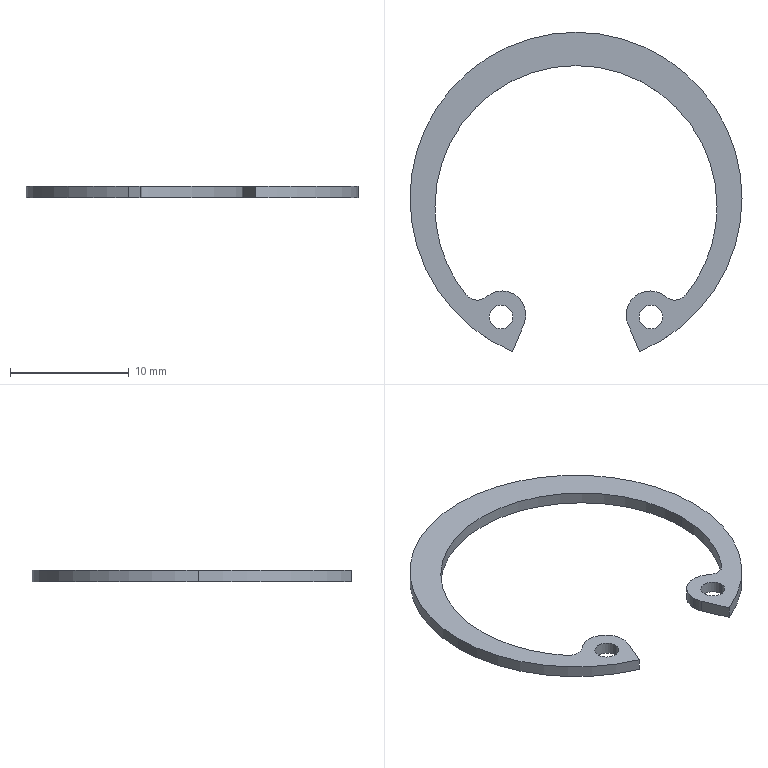Part | SolidWorks | features Extrusion 1 | 1 solid | 19 faces | box 27.9 x 26.838 x 1 mm | volume 169.048 mm3 | cylinder 15 | plane 4 | commonest cylinder face diameters 2 x4 4 x3 23.7 x3 27.9 x3 2.4 x2
STEP:
#1=CARTESIAN_POINT('',(5.298,-9.979,1.));
#2=VERTEX_POINT('',#1);
#3=CARTESIAN_POINT('',(7.298,-9.979,1.));
#4=VERTEX_POINT('',#3);
#5=CARTESIAN_POINT('',(6.298,-9.979,1.));
#6=DIRECTION('',(0.,0.,1.));
#7=DIRECTION('',(-1.,0.,0.));
#8=AXIS2_PLACEMENT_3D('',#5,#6,#7);
#9=CIRCLE('',#8,1.);
#10=EDGE_CURVE('',#2,#4,#9,.T.);
#11=ORIENTED_EDGE('',*,*,#10,.T.);
#12=CARTESIAN_POINT('',(7.298,-9.979,0.));
#13=VERTEX_POINT('',#12);
#14=CARTESIAN_POINT('',(7.298,-9.979,1.));
#15=DIRECTION('',(0.,0.,-1.));
#16=VECTOR('',#15,1000.);
#17=LINE('',#14,#16);
#18=EDGE_CURVE('',#4,#13,#17,.T.);
#19=ORIENTED_EDGE('',*,*,#18,.T.);
#20=CARTESIAN_POINT('',(5.298,-9.979,0.));
#21=VERTEX_POINT('',#20);
#22=CARTESIAN_POINT('',(6.298,-9.979,0.));
#23=DIRECTION('',(0.,0.,1.));
#24=DIRECTION('',(-1.,0.,0.));
#25=AXIS2_PLACEMENT_3D('',#22,#23,#24);
#26=CIRCLE('',#25,1.);
#27=EDGE_CURVE('',#21,#13,#26,.T.);
#28=ORIENTED_EDGE('',*,*,#27,.F.);
#29=CARTESIAN_POINT('',(5.298,-9.979,1.));
#30=DIRECTION('',(0.,0.,-1.));
#31=VECTOR('',#30,1000.);
#32=LINE('',#29,#31);
#33=EDGE_CURVE('',#2,#21,#32,.T.);
#34=ORIENTED_EDGE('',*,*,#33,.F.);
#35=EDGE_LOOP('',(#11,#19,#28,#34));
#36=FACE_OUTER_BOUND('',#35,.T.);
#37=CARTESIAN_POINT('',(6.298,-9.979,1.));
#38=DIRECTION('',(0.,0.,-1.));
#39=DIRECTION('',(-1.,0.,0.));
#40=AXIS2_PLACEMENT_3D('',#37,#38,#39);
#41=CYLINDRICAL_SURFACE('',#40,1.);
#42=ADVANCED_FACE('',(#36),#41,.F.);
#43=CARTESIAN_POINT('',(-7.298,-9.979,1.));
#44=VERTEX_POINT('',#43);
#45=CARTESIAN_POINT('',(-5.298,-9.979,1.));
#46=VERTEX_POINT('',#45);
#47=CARTESIAN_POINT('',(-6.298,-9.979,1.));
#48=DIRECTION('',(0.,0.,1.));
#49=DIRECTION('',(1.,0.,0.));
#50=AXIS2_PLACEMENT_3D('',#47,#48,#49);
#51=CIRCLE('',#50,1.);
#52=EDGE_CURVE('',#44,#46,#51,.T.);
#53=ORIENTED_EDGE('',*,*,#52,.T.);
#54=CARTESIAN_POINT('',(-5.298,-9.979,0.));
#55=VERTEX_POINT('',#54);
#56=CARTESIAN_POINT('',(-5.298,-9.979,1.));
#57=DIRECTION('',(0.,0.,-1.));
#58=VECTOR('',#57,1000.);
#59=LINE('',#56,#58);
#60=EDGE_CURVE('',#46,#55,#59,.T.);
#61=ORIENTED_EDGE('',*,*,#60,.T.);
#62=CARTESIAN_POINT('',(-7.298,-9.979,0.));
#63=VERTEX_POINT('',#62);
#64=CARTESIAN_POINT('',(-6.298,-9.979,0.));
#65=DIRECTION('',(0.,0.,1.));
#66=DIRECTION('',(1.,0.,0.));
#67=AXIS2_PLACEMENT_3D('',#64,#65,#66);
#68=CIRCLE('',#67,1.);
#69=EDGE_CURVE('',#63,#55,#68,.T.);
#70=ORIENTED_EDGE('',*,*,#69,.F.);
#71=CARTESIAN_POINT('',(-7.298,-9.979,1.));
#72=DIRECTION('',(0.,0.,-1.));
#73=VECTOR('',#72,1000.);
#74=LINE('',#71,#73);
#75=EDGE_CURVE('',#44,#63,#74,.T.);
#76=ORIENTED_EDGE('',*,*,#75,.F.);
#77=EDGE_LOOP('',(#53,#61,#70,#76));
#78=FACE_OUTER_BOUND('',#77,.T.);
#79=CARTESIAN_POINT('',(-6.298,-9.979,1.));
#80=DIRECTION('',(0.,0.,-1.));
#81=DIRECTION('',(-1.,0.,0.));
#82=AXIS2_PLACEMENT_3D('',#79,#80,#81);
#83=CYLINDRICAL_SURFACE('',#82,1.);
#84=ADVANCED_FACE('',(#78),#83,.F.);
#85=CARTESIAN_POINT('',(13.95,0.,1.));
#86=VERTEX_POINT('',#85);
#87=CARTESIAN_POINT('',(-13.95,0.,1.));
#88=VERTEX_POINT('',#87);
#89=CARTESIAN_POINT('',(0.,0.,1.));
#90=DIRECTION('',(0.,0.,1.));
#91=DIRECTION('',(1.,0.,0.));
#92=AXIS2_PLACEMENT_3D('',#89,#90,#91);
#93=CIRCLE('',#92,13.95);
#94=EDGE_CURVE('',#86,#88,#93,.T.);
#95=ORIENTED_EDGE('',*,*,#94,.F.);
#96=CARTESIAN_POINT('',(13.95,0.,0.));
#97=VERTEX_POINT('',#96);
#98=CARTESIAN_POINT('',(13.95,0.,1.));
#99=DIRECTION('',(0.,0.,-1.));
#100=VECTOR('',#99,1000.);
#101=LINE('',#98,#100);
#102=EDGE_CURVE('',#86,#97,#101,.T.);
#103=ORIENTED_EDGE('',*,*,#102,.T.);
#104=CARTESIAN_POINT('',(-13.95,0.,0.));
#105=VERTEX_POINT('',#104);
#106=CARTESIAN_POINT('',(0.,0.,0.));
#107=DIRECTION('',(0.,0.,1.));
#108=DIRECTION('',(1.,0.,0.));
#109=AXIS2_PLACEMENT_3D('',#106,#107,#108);
#110=CIRCLE('',#109,13.95);
#111=EDGE_CURVE('',#97,#105,#110,.T.);
#112=ORIENTED_EDGE('',*,*,#111,.T.);
#113=CARTESIAN_POINT('',(-13.95,0.,1.));
#114=DIRECTION('',(0.,0.,-1.));
#115=VECTOR('',#114,1000.);
#116=LINE('',#113,#115);
#117=EDGE_CURVE('',#88,#105,#116,.T.);
#118=ORIENTED_EDGE('',*,*,#117,.F.);
#119=EDGE_LOOP('',(#95,#103,#112,#118));
#120=FACE_OUTER_BOUND('',#119,.T.);
#121=CARTESIAN_POINT('',(0.,0.,1.));
#122=DIRECTION('',(0.,0.,-1.));
#123=DIRECTION('',(-1.,0.,0.));
#124=AXIS2_PLACEMENT_3D('',#121,#122,#123);
#125=CYLINDRICAL_SURFACE('',#124,13.95);
#126=ADVANCED_FACE('',(#120),#125,.T.);
#127=CARTESIAN_POINT('',(-5.338,-12.888,1.));
#128=VERTEX_POINT('',#127);
#129=CARTESIAN_POINT('',(0.,0.,1.));
#130=DIRECTION('',(0.,0.,1.));
#131=DIRECTION('',(1.,0.,0.));
#132=AXIS2_PLACEMENT_3D('',#129,#130,#131);
#133=CIRCLE('',#132,13.95);
#134=EDGE_CURVE('',#88,#128,#133,.T.);
#135=ORIENTED_EDGE('',*,*,#134,.F.);
#136=ORIENTED_EDGE('',*,*,#117,.T.);
#137=CARTESIAN_POINT('',(-5.338,-12.888,0.));
#138=VERTEX_POINT('',#137);
#139=CARTESIAN_POINT('',(0.,0.,0.));
#140=DIRECTION('',(0.,0.,1.));
#141=DIRECTION('',(1.,0.,0.));
#142=AXIS2_PLACEMENT_3D('',#139,#140,#141);
#143=CIRCLE('',#142,13.95);
#144=EDGE_CURVE('',#105,#138,#143,.T.);
#145=ORIENTED_EDGE('',*,*,#144,.T.);
#146=CARTESIAN_POINT('',(-5.338,-12.888,1.));
#147=DIRECTION('',(0.,0.,-1.));
#148=VECTOR('',#147,1000.);
#149=LINE('',#146,#148);
#150=EDGE_CURVE('',#128,#138,#149,.T.);
#151=ORIENTED_EDGE('',*,*,#150,.F.);
#152=EDGE_LOOP('',(#135,#136,#145,#151));
#153=FACE_OUTER_BOUND('',#152,.T.);
#154=CARTESIAN_POINT('',(0.,0.,1.));
#155=DIRECTION('',(0.,0.,-1.));
#156=DIRECTION('',(-1.,0.,0.));
#157=AXIS2_PLACEMENT_3D('',#154,#155,#156);
#158=CYLINDRICAL_SURFACE('',#157,13.95);
#159=ADVANCED_FACE('',(#153),#158,.T.);
#160=CARTESIAN_POINT('',(4.217,-9.782,1.));
#161=VERTEX_POINT('',#160);
#162=CARTESIAN_POINT('',(4.369,-10.547,1.));
#163=VERTEX_POINT('',#162);
#164=CARTESIAN_POINT('',(6.217,-9.782,1.));
#165=DIRECTION('',(0.,0.,1.));
#166=DIRECTION('',(-1.,0.,0.));
#167=AXIS2_PLACEMENT_3D('',#164,#165,#166);
#168=CIRCLE('',#167,2.);
#169=EDGE_CURVE('',#161,#163,#168,.T.);
#170=ORIENTED_EDGE('',*,*,#169,.F.);
#171=CARTESIAN_POINT('',(4.217,-9.782,0.));
#172=VERTEX_POINT('',#171);
#173=CARTESIAN_POINT('',(4.217,-9.782,1.));
#174=DIRECTION('',(0.,0.,-1.));
#175=VECTOR('',#174,1000.);
#176=LINE('',#173,#175);
#177=EDGE_CURVE('',#161,#172,#176,.T.);
#178=ORIENTED_EDGE('',*,*,#177,.T.);
#179=CARTESIAN_POINT('',(4.369,-10.547,0.));
#180=VERTEX_POINT('',#179);
#181=CARTESIAN_POINT('',(6.217,-9.782,0.));
#182=DIRECTION('',(0.,0.,1.));
#183=DIRECTION('',(-1.,0.,0.));
#184=AXIS2_PLACEMENT_3D('',#181,#182,#183);
#185=CIRCLE('',#184,2.);
#186=EDGE_CURVE('',#172,#180,#185,.T.);
#187=ORIENTED_EDGE('',*,*,#186,.T.);
#188=CARTESIAN_POINT('',(4.369,-10.547,1.));
#189=DIRECTION('',(0.,0.,-1.));
#190=VECTOR('',#189,1000.);
#191=LINE('',#188,#190);
#192=EDGE_CURVE('',#163,#180,#191,.T.);
#193=ORIENTED_EDGE('',*,*,#192,.F.);
#194=EDGE_LOOP('',(#170,#178,#187,#193));
#195=FACE_OUTER_BOUND('',#194,.T.);
#196=CARTESIAN_POINT('',(6.217,-9.782,1.));
#197=DIRECTION('',(0.,0.,-1.));
#198=DIRECTION('',(-1.,0.,0.));
#199=AXIS2_PLACEMENT_3D('',#196,#197,#198);
#200=CYLINDRICAL_SURFACE('',#199,2.);
#201=ADVANCED_FACE('',(#195),#200,.T.);
#202=CARTESIAN_POINT('',(11.85,-0.7,1.));
#203=VERTEX_POINT('',#202);
#204=CARTESIAN_POINT('',(9.246,-8.112,1.));
#205=VERTEX_POINT('',#204);
#206=CARTESIAN_POINT('',(0.,-0.7,1.));
#207=DIRECTION('',(0.,0.,-1.));
#208=DIRECTION('',(1.,0.,0.));
#209=AXIS2_PLACEMENT_3D('',#206,#207,#208);
#210=CIRCLE('',#209,11.85);
#211=EDGE_CURVE('',#203,#205,#210,.T.);
#212=ORIENTED_EDGE('',*,*,#211,.F.);
#213=CARTESIAN_POINT('',(11.85,-0.7,0.));
#214=VERTEX_POINT('',#213);
#215=CARTESIAN_POINT('',(11.85,-0.7,1.));
#216=DIRECTION('',(0.,0.,-1.));
#217=VECTOR('',#216,1000.);
#218=LINE('',#215,#217);
#219=EDGE_CURVE('',#203,#214,#218,.T.);
#220=ORIENTED_EDGE('',*,*,#219,.T.);
#221=CARTESIAN_POINT('',(9.246,-8.112,0.));
#222=VERTEX_POINT('',#221);
#223=CARTESIAN_POINT('',(0.,-0.7,0.));
#224=DIRECTION('',(0.,0.,-1.));
#225=DIRECTION('',(1.,0.,0.));
#226=AXIS2_PLACEMENT_3D('',#223,#224,#225);
#227=CIRCLE('',#226,11.85);
#228=EDGE_CURVE('',#214,#222,#227,.T.);
#229=ORIENTED_EDGE('',*,*,#228,.T.);
#230=CARTESIAN_POINT('',(9.246,-8.112,1.));
#231=DIRECTION('',(0.,0.,-1.));
#232=VECTOR('',#231,1000.);
#233=LINE('',#230,#232);
#234=EDGE_CURVE('',#205,#222,#233,.T.);
#235=ORIENTED_EDGE('',*,*,#234,.F.);
#236=EDGE_LOOP('',(#212,#220,#229,#235));
#237=FACE_OUTER_BOUND('',#236,.T.);
#238=CARTESIAN_POINT('',(0.,-0.7,1.));
#239=DIRECTION('',(0.,0.,-1.));
#240=DIRECTION('',(-1.,0.,0.));
#241=AXIS2_PLACEMENT_3D('',#238,#239,#240);
#242=CYLINDRICAL_SURFACE('',#241,11.85);
#243=ADVANCED_FACE('',(#237),#242,.F.);
#244=ORIENTED_EDGE('',*,*,#219,.F.);
#245=CARTESIAN_POINT('',(-11.85,-0.7,1.));
#246=VERTEX_POINT('',#245);
#247=CARTESIAN_POINT('',(0.,-0.7,1.));
#248=DIRECTION('',(0.,0.,-1.));
#249=DIRECTION('',(1.,0.,0.));
#250=AXIS2_PLACEMENT_3D('',#247,#248,#249);
#251=CIRCLE('',#250,11.85);
#252=EDGE_CURVE('',#246,#203,#251,.T.);
#253=ORIENTED_EDGE('',*,*,#252,.F.);
#254=CARTESIAN_POINT('',(-11.85,-0.7,0.));
#255=VERTEX_POINT('',#254);
#256=CARTESIAN_POINT('',(-11.85,-0.7,1.));
#257=DIRECTION('',(0.,0.,-1.));
#258=VECTOR('',#257,1000.);
#259=LINE('',#256,#258);
#260=EDGE_CURVE('',#246,#255,#259,.T.);
#261=ORIENTED_EDGE('',*,*,#260,.T.);
#262=CARTESIAN_POINT('',(0.,-0.7,0.));
#263=DIRECTION('',(0.,0.,-1.));
#264=DIRECTION('',(1.,0.,0.));
#265=AXIS2_PLACEMENT_3D('',#262,#263,#264);
#266=CIRCLE('',#265,11.85);
#267=EDGE_CURVE('',#255,#214,#266,.T.);
#268=ORIENTED_EDGE('',*,*,#267,.T.);
#269=EDGE_LOOP('',(#244,#253,#261,#268));
#270=FACE_OUTER_BOUND('',#269,.T.);
#271=CARTESIAN_POINT('',(0.,-0.7,1.));
#272=DIRECTION('',(0.,0.,-1.));
#273=DIRECTION('',(-1.,0.,0.));
#274=AXIS2_PLACEMENT_3D('',#271,#272,#273);
#275=CYLINDRICAL_SURFACE('',#274,11.85);
#276=ADVANCED_FACE('',(#270),#275,.F.);
#277=ORIENTED_EDGE('',*,*,#52,.F.);
#278=CARTESIAN_POINT('',(-6.298,-9.979,1.));
#279=DIRECTION('',(0.,0.,1.));
#280=DIRECTION('',(1.,0.,0.));
#281=AXIS2_PLACEMENT_3D('',#278,#279,#280);
#282=CIRCLE('',#281,1.);
#283=EDGE_CURVE('',#46,#44,#282,.T.);
#284=ORIENTED_EDGE('',*,*,#283,.F.);
#285=EDGE_LOOP('',(#277,#284));
#286=FACE_BOUND('',#285,.T.);
#287=CARTESIAN_POINT('',(-4.369,-10.547,1.));
#288=VERTEX_POINT('',#287);
#289=CARTESIAN_POINT('',(-7.525,-8.269,1.));
#290=VERTEX_POINT('',#289);
#291=CARTESIAN_POINT('',(-6.217,-9.782,1.));
#292=DIRECTION('',(0.,0.,1.));
#293=DIRECTION('',(1.,0.,0.));
#294=AXIS2_PLACEMENT_3D('',#291,#292,#293);
#295=CIRCLE('',#294,2.);
#296=EDGE_CURVE('',#288,#290,#295,.T.);
#297=ORIENTED_EDGE('',*,*,#296,.T.);
#298=CARTESIAN_POINT('',(-9.246,-8.112,1.));
#299=VERTEX_POINT('',#298);
#300=CARTESIAN_POINT('',(-8.31,-7.361,1.));
#301=DIRECTION('',(0.,0.,-1.));
#302=DIRECTION('',(-1.,0.,0.));
#303=AXIS2_PLACEMENT_3D('',#300,#301,#302);
#304=CIRCLE('',#303,1.2);
#305=EDGE_CURVE('',#290,#299,#304,.T.);
#306=ORIENTED_EDGE('',*,*,#305,.T.);
#307=CARTESIAN_POINT('',(0.,-0.7,1.));
#308=DIRECTION('',(0.,0.,-1.));
#309=DIRECTION('',(1.,0.,0.));
#310=AXIS2_PLACEMENT_3D('',#307,#308,#309);
#311=CIRCLE('',#310,11.85);
#312=EDGE_CURVE('',#299,#246,#311,.T.);
#313=ORIENTED_EDGE('',*,*,#312,.T.);
#314=ORIENTED_EDGE('',*,*,#252,.T.);
#315=ORIENTED_EDGE('',*,*,#211,.T.);
#316=CARTESIAN_POINT('',(7.525,-8.269,1.));
#317=VERTEX_POINT('',#316);
#318=CARTESIAN_POINT('',(8.31,-7.361,1.));
#319=DIRECTION('',(0.,0.,-1.));
#320=DIRECTION('',(1.,0.,0.));
#321=AXIS2_PLACEMENT_3D('',#318,#319,#320);
#322=CIRCLE('',#321,1.2);
#323=EDGE_CURVE('',#205,#317,#322,.T.);
#324=ORIENTED_EDGE('',*,*,#323,.T.);
#325=CARTESIAN_POINT('',(6.217,-9.782,1.));
#326=DIRECTION('',(0.,0.,1.));
#327=DIRECTION('',(-1.,0.,0.));
#328=AXIS2_PLACEMENT_3D('',#325,#326,#327);
#329=CIRCLE('',#328,2.);
#330=EDGE_CURVE('',#317,#161,#329,.T.);
#331=ORIENTED_EDGE('',*,*,#330,.T.);
#332=ORIENTED_EDGE('',*,*,#169,.T.);
#333=CARTESIAN_POINT('',(5.338,-12.888,1.));
#334=VERTEX_POINT('',#333);
#335=CARTESIAN_POINT('',(4.369,-10.547,1.));
#336=DIRECTION('',(0.3827,-0.9239,0.));
#337=VECTOR('',#336,1000.);
#338=LINE('',#335,#337);
#339=EDGE_CURVE('',#163,#334,#338,.T.);
#340=ORIENTED_EDGE('',*,*,#339,.T.);
#341=CARTESIAN_POINT('',(0.,0.,1.));
#342=DIRECTION('',(0.,0.,1.));
#343=DIRECTION('',(1.,0.,0.));
#344=AXIS2_PLACEMENT_3D('',#341,#342,#343);
#345=CIRCLE('',#344,13.95);
#346=EDGE_CURVE('',#334,#86,#345,.T.);
#347=ORIENTED_EDGE('',*,*,#346,.T.);
#348=ORIENTED_EDGE('',*,*,#94,.T.);
#349=ORIENTED_EDGE('',*,*,#134,.T.);
#350=CARTESIAN_POINT('',(-4.369,-10.547,1.));
#351=DIRECTION('',(0.3827,0.9239,0.));
#352=VECTOR('',#351,1000.);
#353=LINE('',#350,#352);
#354=EDGE_CURVE('',#128,#288,#353,.T.);
#355=ORIENTED_EDGE('',*,*,#354,.T.);
#356=EDGE_LOOP('',(#297,#306,#313,#314,#315,#324,#331,#332,#340,#347,#348,#349,#355));
#357=FACE_OUTER_BOUND('',#356,.T.);
#358=ORIENTED_EDGE('',*,*,#10,.F.);
#359=CARTESIAN_POINT('',(6.298,-9.979,1.));
#360=DIRECTION('',(0.,0.,1.));
#361=DIRECTION('',(-1.,0.,0.));
#362=AXIS2_PLACEMENT_3D('',#359,#360,#361);
#363=CIRCLE('',#362,1.);
#364=EDGE_CURVE('',#4,#2,#363,.T.);
#365=ORIENTED_EDGE('',*,*,#364,.F.);
#366=EDGE_LOOP('',(#358,#365));
#367=FACE_BOUND('',#366,.T.);
#368=CARTESIAN_POINT('',(-6.217,-9.782,1.));
#369=DIRECTION('',(0.,0.,1.));
#370=DIRECTION('',(1.,0.,0.));
#371=AXIS2_PLACEMENT_3D('',#368,#369,#370);
#372=PLANE('',#371);
#373=ADVANCED_FACE('',(#286,#357,#367),#372,.T.);
#374=CARTESIAN_POINT('',(-4.369,-10.547,0.));
#375=VERTEX_POINT('',#374);
#376=CARTESIAN_POINT('',(-7.525,-8.269,0.));
#377=VERTEX_POINT('',#376);
#378=CARTESIAN_POINT('',(-6.217,-9.782,0.));
#379=DIRECTION('',(0.,0.,1.));
#380=DIRECTION('',(1.,0.,0.));
#381=AXIS2_PLACEMENT_3D('',#378,#379,#380);
#382=CIRCLE('',#381,2.);
#383=EDGE_CURVE('',#375,#377,#382,.T.);
#384=ORIENTED_EDGE('',*,*,#383,.F.);
#385=CARTESIAN_POINT('',(-4.369,-10.547,0.));
#386=DIRECTION('',(0.3827,0.9239,0.));
#387=VECTOR('',#386,1000.);
#388=LINE('',#385,#387);
#389=EDGE_CURVE('',#138,#375,#388,.T.);
#390=ORIENTED_EDGE('',*,*,#389,.F.);
#391=ORIENTED_EDGE('',*,*,#144,.F.);
#392=ORIENTED_EDGE('',*,*,#111,.F.);
#393=CARTESIAN_POINT('',(5.338,-12.888,0.));
#394=VERTEX_POINT('',#393);
#395=CARTESIAN_POINT('',(0.,0.,0.));
#396=DIRECTION('',(0.,0.,1.));
#397=DIRECTION('',(1.,0.,0.));
#398=AXIS2_PLACEMENT_3D('',#395,#396,#397);
#399=CIRCLE('',#398,13.95);
#400=EDGE_CURVE('',#394,#97,#399,.T.);
#401=ORIENTED_EDGE('',*,*,#400,.F.);
#402=CARTESIAN_POINT('',(4.369,-10.547,0.));
#403=DIRECTION('',(0.3827,-0.9239,0.));
#404=VECTOR('',#403,1000.);
#405=LINE('',#402,#404);
#406=EDGE_CURVE('',#180,#394,#405,.T.);
#407=ORIENTED_EDGE('',*,*,#406,.F.);
#408=ORIENTED_EDGE('',*,*,#186,.F.);
#409=CARTESIAN_POINT('',(7.525,-8.269,0.));
#410=VERTEX_POINT('',#409);
#411=CARTESIAN_POINT('',(6.217,-9.782,0.));
#412=DIRECTION('',(0.,0.,1.));
#413=DIRECTION('',(-1.,0.,0.));
#414=AXIS2_PLACEMENT_3D('',#411,#412,#413);
#415=CIRCLE('',#414,2.);
#416=EDGE_CURVE('',#410,#172,#415,.T.);
#417=ORIENTED_EDGE('',*,*,#416,.F.);
#418=CARTESIAN_POINT('',(8.31,-7.361,0.));
#419=DIRECTION('',(0.,0.,-1.));
#420=DIRECTION('',(1.,0.,0.));
#421=AXIS2_PLACEMENT_3D('',#418,#419,#420);
#422=CIRCLE('',#421,1.2);
#423=EDGE_CURVE('',#222,#410,#422,.T.);
#424=ORIENTED_EDGE('',*,*,#423,.F.);
#425=ORIENTED_EDGE('',*,*,#228,.F.);
#426=ORIENTED_EDGE('',*,*,#267,.F.);
#427=CARTESIAN_POINT('',(-9.246,-8.112,0.));
#428=VERTEX_POINT('',#427);
#429=CARTESIAN_POINT('',(0.,-0.7,0.));
#430=DIRECTION('',(0.,0.,-1.));
#431=DIRECTION('',(1.,0.,0.));
#432=AXIS2_PLACEMENT_3D('',#429,#430,#431);
#433=CIRCLE('',#432,11.85);
#434=EDGE_CURVE('',#428,#255,#433,.T.);
#435=ORIENTED_EDGE('',*,*,#434,.F.);
#436=CARTESIAN_POINT('',(-8.31,-7.361,0.));
#437=DIRECTION('',(0.,0.,-1.));
#438=DIRECTION('',(-1.,0.,0.));
#439=AXIS2_PLACEMENT_3D('',#436,#437,#438);
#440=CIRCLE('',#439,1.2);
#441=EDGE_CURVE('',#377,#428,#440,.T.);
#442=ORIENTED_EDGE('',*,*,#441,.F.);
#443=EDGE_LOOP('',(#384,#390,#391,#392,#401,#407,#408,#417,#424,#425,#426,#435,#442));
#444=FACE_OUTER_BOUND('',#443,.T.);
#445=ORIENTED_EDGE('',*,*,#69,.T.);
#446=CARTESIAN_POINT('',(-6.298,-9.979,0.));
#447=DIRECTION('',(0.,0.,1.));
#448=DIRECTION('',(1.,0.,0.));
#449=AXIS2_PLACEMENT_3D('',#446,#447,#448);
#450=CIRCLE('',#449,1.);
#451=EDGE_CURVE('',#55,#63,#450,.T.);
#452=ORIENTED_EDGE('',*,*,#451,.T.);
#453=EDGE_LOOP('',(#445,#452));
#454=FACE_BOUND('',#453,.T.);
#455=ORIENTED_EDGE('',*,*,#27,.T.);
#456=CARTESIAN_POINT('',(6.298,-9.979,0.));
#457=DIRECTION('',(0.,0.,1.));
#458=DIRECTION('',(-1.,0.,0.));
#459=AXIS2_PLACEMENT_3D('',#456,#457,#458);
#460=CIRCLE('',#459,1.);
#461=EDGE_CURVE('',#13,#21,#460,.T.);
#462=ORIENTED_EDGE('',*,*,#461,.T.);
#463=EDGE_LOOP('',(#455,#462));
#464=FACE_BOUND('',#463,.T.);
#465=CARTESIAN_POINT('',(-6.217,-9.782,0.));
#466=DIRECTION('',(0.,0.,1.));
#467=DIRECTION('',(1.,0.,0.));
#468=AXIS2_PLACEMENT_3D('',#465,#466,#467);
#469=PLANE('',#468);
#470=ADVANCED_FACE('',(#444,#454,#464),#469,.F.);
#471=ORIENTED_EDGE('',*,*,#383,.T.);
#472=CARTESIAN_POINT('',(-7.525,-8.269,1.));
#473=DIRECTION('',(0.,0.,-1.));
#474=VECTOR('',#473,1000.);
#475=LINE('',#472,#474);
#476=EDGE_CURVE('',#290,#377,#475,.T.);
#477=ORIENTED_EDGE('',*,*,#476,.F.);
#478=ORIENTED_EDGE('',*,*,#296,.F.);
#479=CARTESIAN_POINT('',(-4.369,-10.547,1.));
#480=DIRECTION('',(0.,0.,-1.));
#481=VECTOR('',#480,1000.);
#482=LINE('',#479,#481);
#483=EDGE_CURVE('',#288,#375,#482,.T.);
#484=ORIENTED_EDGE('',*,*,#483,.T.);
#485=EDGE_LOOP('',(#471,#477,#478,#484));
#486=FACE_OUTER_BOUND('',#485,.T.);
#487=CARTESIAN_POINT('',(-6.217,-9.782,1.));
#488=DIRECTION('',(0.,0.,-1.));
#489=DIRECTION('',(-1.,0.,0.));
#490=AXIS2_PLACEMENT_3D('',#487,#488,#489);
#491=CYLINDRICAL_SURFACE('',#490,2.);
#492=ADVANCED_FACE('',(#486),#491,.T.);
#493=ORIENTED_EDGE('',*,*,#441,.T.);
#494=CARTESIAN_POINT('',(-9.246,-8.112,1.));
#495=DIRECTION('',(0.,0.,-1.));
#496=VECTOR('',#495,1000.);
#497=LINE('',#494,#496);
#498=EDGE_CURVE('',#299,#428,#497,.T.);
#499=ORIENTED_EDGE('',*,*,#498,.F.);
#500=ORIENTED_EDGE('',*,*,#305,.F.);
#501=ORIENTED_EDGE('',*,*,#476,.T.);
#502=EDGE_LOOP('',(#493,#499,#500,#501));
#503=FACE_OUTER_BOUND('',#502,.T.);
#504=CARTESIAN_POINT('',(-8.31,-7.361,1.));
#505=DIRECTION('',(0.,0.,-1.));
#506=DIRECTION('',(-1.,0.,0.));
#507=AXIS2_PLACEMENT_3D('',#504,#505,#506);
#508=CYLINDRICAL_SURFACE('',#507,1.2);
#509=ADVANCED_FACE('',(#503),#508,.F.);
#510=ORIENTED_EDGE('',*,*,#260,.F.);
#511=ORIENTED_EDGE('',*,*,#312,.F.);
#512=ORIENTED_EDGE('',*,*,#498,.T.);
#513=ORIENTED_EDGE('',*,*,#434,.T.);
#514=EDGE_LOOP('',(#510,#511,#512,#513));
#515=FACE_OUTER_BOUND('',#514,.T.);
#516=CARTESIAN_POINT('',(0.,-0.7,1.));
#517=DIRECTION('',(0.,0.,-1.));
#518=DIRECTION('',(-1.,0.,0.));
#519=AXIS2_PLACEMENT_3D('',#516,#517,#518);
#520=CYLINDRICAL_SURFACE('',#519,11.85);
#521=ADVANCED_FACE('',(#515),#520,.F.);
#522=ORIENTED_EDGE('',*,*,#423,.T.);
#523=CARTESIAN_POINT('',(7.525,-8.269,1.));
#524=DIRECTION('',(0.,0.,-1.));
#525=VECTOR('',#524,1000.);
#526=LINE('',#523,#525);
#527=EDGE_CURVE('',#317,#410,#526,.T.);
#528=ORIENTED_EDGE('',*,*,#527,.F.);
#529=ORIENTED_EDGE('',*,*,#323,.F.);
#530=ORIENTED_EDGE('',*,*,#234,.T.);
#531=EDGE_LOOP('',(#522,#528,#529,#530));
#532=FACE_OUTER_BOUND('',#531,.T.);
#533=CARTESIAN_POINT('',(8.31,-7.361,1.));
#534=DIRECTION('',(0.,0.,-1.));
#535=DIRECTION('',(-1.,0.,0.));
#536=AXIS2_PLACEMENT_3D('',#533,#534,#535);
#537=CYLINDRICAL_SURFACE('',#536,1.2);
#538=ADVANCED_FACE('',(#532),#537,.F.);
#539=ORIENTED_EDGE('',*,*,#177,.F.);
#540=ORIENTED_EDGE('',*,*,#330,.F.);
#541=ORIENTED_EDGE('',*,*,#527,.T.);
#542=ORIENTED_EDGE('',*,*,#416,.T.);
#543=EDGE_LOOP('',(#539,#540,#541,#542));
#544=FACE_OUTER_BOUND('',#543,.T.);
#545=CARTESIAN_POINT('',(6.217,-9.782,1.));
#546=DIRECTION('',(0.,0.,-1.));
#547=DIRECTION('',(-1.,0.,0.));
#548=AXIS2_PLACEMENT_3D('',#545,#546,#547);
#549=CYLINDRICAL_SURFACE('',#548,2.);
#550=ADVANCED_FACE('',(#544),#549,.T.);
#551=ORIENTED_EDGE('',*,*,#406,.T.);
#552=CARTESIAN_POINT('',(5.338,-12.888,1.));
#553=DIRECTION('',(0.,0.,-1.));
#554=VECTOR('',#553,1000.);
#555=LINE('',#552,#554);
#556=EDGE_CURVE('',#334,#394,#555,.T.);
#557=ORIENTED_EDGE('',*,*,#556,.F.);
#558=ORIENTED_EDGE('',*,*,#339,.F.);
#559=ORIENTED_EDGE('',*,*,#192,.T.);
#560=EDGE_LOOP('',(#551,#557,#558,#559));
#561=FACE_OUTER_BOUND('',#560,.T.);
#562=CARTESIAN_POINT('',(4.369,-10.547,1.));
#563=DIRECTION('',(0.9239,0.3827,0.));
#564=DIRECTION('',(-0.3827,0.9239,0.));
#565=AXIS2_PLACEMENT_3D('',#562,#563,#564);
#566=PLANE('',#565);
#567=ADVANCED_FACE('',(#561),#566,.F.);
#568=ORIENTED_EDGE('',*,*,#102,.F.);
#569=ORIENTED_EDGE('',*,*,#346,.F.);
#570=ORIENTED_EDGE('',*,*,#556,.T.);
#571=ORIENTED_EDGE('',*,*,#400,.T.);
#572=EDGE_LOOP('',(#568,#569,#570,#571));
#573=FACE_OUTER_BOUND('',#572,.T.);
#574=CARTESIAN_POINT('',(0.,0.,1.));
#575=DIRECTION('',(0.,0.,-1.));
#576=DIRECTION('',(-1.,0.,0.));
#577=AXIS2_PLACEMENT_3D('',#574,#575,#576);
#578=CYLINDRICAL_SURFACE('',#577,13.95);
#579=ADVANCED_FACE('',(#573),#578,.T.);
#580=ORIENTED_EDGE('',*,*,#389,.T.);
#581=ORIENTED_EDGE('',*,*,#483,.F.);
#582=ORIENTED_EDGE('',*,*,#354,.F.);
#583=ORIENTED_EDGE('',*,*,#150,.T.);
#584=EDGE_LOOP('',(#580,#581,#582,#583));
#585=FACE_OUTER_BOUND('',#584,.T.);
#586=CARTESIAN_POINT('',(-4.369,-10.547,1.));
#587=DIRECTION('',(-0.9239,0.3827,0.));
#588=DIRECTION('',(-0.3827,-0.9239,0.));
#589=AXIS2_PLACEMENT_3D('',#586,#587,#588);
#590=PLANE('',#589);
#591=ADVANCED_FACE('',(#585),#590,.F.);
#592=ORIENTED_EDGE('',*,*,#60,.F.);
#593=ORIENTED_EDGE('',*,*,#283,.T.);
#594=ORIENTED_EDGE('',*,*,#75,.T.);
#595=ORIENTED_EDGE('',*,*,#451,.F.);
#596=EDGE_LOOP('',(#592,#593,#594,#595));
#597=FACE_OUTER_BOUND('',#596,.T.);
#598=CARTESIAN_POINT('',(-6.298,-9.979,1.));
#599=DIRECTION('',(0.,0.,-1.));
#600=DIRECTION('',(-1.,0.,0.));
#601=AXIS2_PLACEMENT_3D('',#598,#599,#600);
#602=CYLINDRICAL_SURFACE('',#601,1.);
#603=ADVANCED_FACE('',(#597),#602,.F.);
#604=ORIENTED_EDGE('',*,*,#18,.F.);
#605=ORIENTED_EDGE('',*,*,#364,.T.);
#606=ORIENTED_EDGE('',*,*,#33,.T.);
#607=ORIENTED_EDGE('',*,*,#461,.F.);
#608=EDGE_LOOP('',(#604,#605,#606,#607));
#609=FACE_OUTER_BOUND('',#608,.T.);
#610=CARTESIAN_POINT('',(6.298,-9.979,1.));
#611=DIRECTION('',(0.,0.,-1.));
#612=DIRECTION('',(-1.,0.,0.));
#613=AXIS2_PLACEMENT_3D('',#610,#611,#612);
#614=CYLINDRICAL_SURFACE('',#613,1.);
#615=ADVANCED_FACE('',(#609),#614,.F.);
#616=CLOSED_SHELL('',(#42,#84,#126,#159,#201,#243,#276,#373,#470,#492,#509,#521,#538,#550,#567,#579,#591,#603,#615));
#617=MANIFOLD_SOLID_BREP('',#616);
#618=CARTESIAN_POINT('',(0.,0.,0.));
#619=DIRECTION('',(0.,0.,1.));
#620=DIRECTION('',(1.,0.,0.));
#621=AXIS2_PLACEMENT_3D('',#618,#619,#620);
#622=(LENGTH_UNIT()NAMED_UNIT(*)SI_UNIT(.MILLI.,.METRE.));
#623=UNCERTAINTY_MEASURE_WITH_UNIT(LENGTH_MEASURE(0.00001),#622,'','');
#624=(NAMED_UNIT(*)PLANE_ANGLE_UNIT()SI_UNIT($,.RADIAN.));
#625=(NAMED_UNIT(*)SI_UNIT($,.STERADIAN.)SOLID_ANGLE_UNIT());
#626=(GEOMETRIC_REPRESENTATION_CONTEXT(3)GLOBAL_UNCERTAINTY_ASSIGNED_CONTEXT((#623))GLOBAL_UNIT_ASSIGNED_CONTEXT((#622,#624,#625))REPRESENTATION_CONTEXT('',''));
#627=ADVANCED_BREP_SHAPE_REPRESENTATION('',(#617,#621),#626);